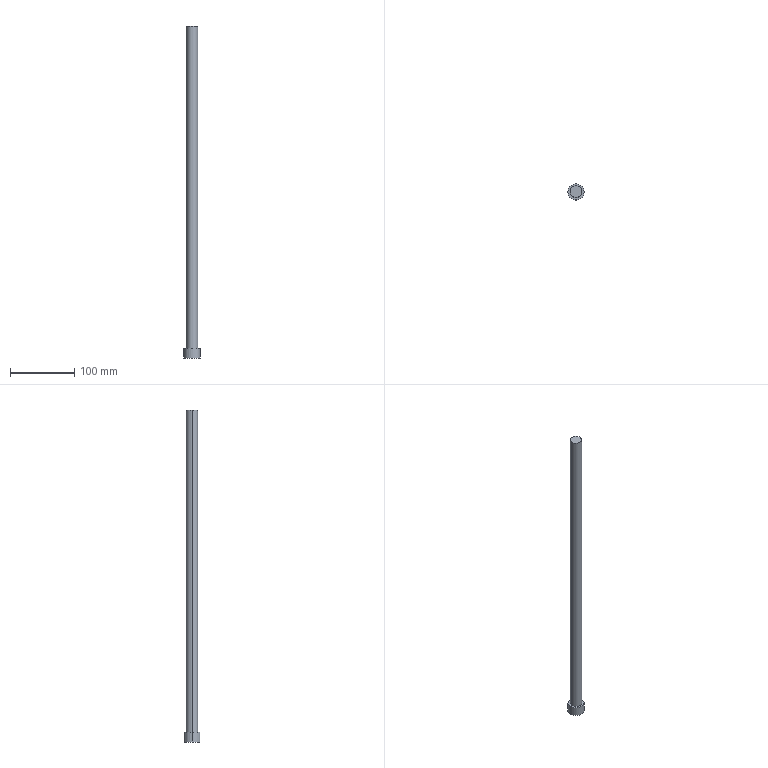Part | SolidWorks | features Extrusion 1, ICE 1 | 1 solid | 7 faces | box 25 x 25 x 515 mm | volume 134598 mm3 | cylinder 4 | plane 3 | commonest cylinder face diameters 18 x2 25 x2
STEP:
#1=CARTESIAN_POINT('',(-12.5,0.,-15.));
#2=VERTEX_POINT('',#1);
#3=CARTESIAN_POINT('',(12.5,0.,-15.));
#4=VERTEX_POINT('',#3);
#5=CARTESIAN_POINT('',(0.,0.,-15.));
#6=DIRECTION('',(0.,0.,-1.));
#7=DIRECTION('',(-1.,0.,0.));
#8=AXIS2_PLACEMENT_3D('',#5,#6,#7);
#9=CIRCLE('',#8,12.5);
#10=EDGE_CURVE('',#2,#4,#9,.T.);
#11=ORIENTED_EDGE('',*,*,#10,.F.);
#12=CARTESIAN_POINT('',(-12.5,0.,0.));
#13=VERTEX_POINT('',#12);
#14=CARTESIAN_POINT('',(-12.5,0.,-15.));
#15=DIRECTION('',(0.,0.,1.));
#16=VECTOR('',#15,1000.);
#17=LINE('',#14,#16);
#18=EDGE_CURVE('',#2,#13,#17,.T.);
#19=ORIENTED_EDGE('',*,*,#18,.T.);
#20=CARTESIAN_POINT('',(12.5,0.,0.));
#21=VERTEX_POINT('',#20);
#22=CARTESIAN_POINT('',(0.,0.,0.));
#23=DIRECTION('',(0.,0.,-1.));
#24=DIRECTION('',(-1.,0.,0.));
#25=AXIS2_PLACEMENT_3D('',#22,#23,#24);
#26=CIRCLE('',#25,12.5);
#27=EDGE_CURVE('',#13,#21,#26,.T.);
#28=ORIENTED_EDGE('',*,*,#27,.T.);
#29=CARTESIAN_POINT('',(12.5,0.,-15.));
#30=DIRECTION('',(0.,0.,1.));
#31=VECTOR('',#30,1000.);
#32=LINE('',#29,#31);
#33=EDGE_CURVE('',#4,#21,#32,.T.);
#34=ORIENTED_EDGE('',*,*,#33,.F.);
#35=EDGE_LOOP('',(#11,#19,#28,#34));
#36=FACE_OUTER_BOUND('',#35,.T.);
#37=CARTESIAN_POINT('',(0.,0.,-15.));
#38=DIRECTION('',(0.,0.,1.));
#39=DIRECTION('',(1.,0.,0.));
#40=AXIS2_PLACEMENT_3D('',#37,#38,#39);
#41=CYLINDRICAL_SURFACE('',#40,12.5);
#42=ADVANCED_FACE('',(#36),#41,.T.);
#43=CARTESIAN_POINT('',(9.,0.,500.));
#44=VERTEX_POINT('',#43);
#45=CARTESIAN_POINT('',(-9.,0.,500.));
#46=VERTEX_POINT('',#45);
#47=CARTESIAN_POINT('',(0.,0.,500.));
#48=DIRECTION('',(0.,0.,1.));
#49=DIRECTION('',(1.,0.,0.));
#50=AXIS2_PLACEMENT_3D('',#47,#48,#49);
#51=CIRCLE('',#50,9.);
#52=EDGE_CURVE('',#44,#46,#51,.T.);
#53=ORIENTED_EDGE('',*,*,#52,.F.);
#54=CARTESIAN_POINT('',(9.,0.,0.));
#55=VERTEX_POINT('',#54);
#56=CARTESIAN_POINT('',(9.,0.,500.));
#57=DIRECTION('',(0.,0.,-1.));
#58=VECTOR('',#57,1000.);
#59=LINE('',#56,#58);
#60=EDGE_CURVE('',#44,#55,#59,.T.);
#61=ORIENTED_EDGE('',*,*,#60,.T.);
#62=CARTESIAN_POINT('',(-9.,0.,0.));
#63=VERTEX_POINT('',#62);
#64=CARTESIAN_POINT('',(0.,0.,0.));
#65=DIRECTION('',(0.,0.,-1.));
#66=DIRECTION('',(-1.,0.,0.));
#67=AXIS2_PLACEMENT_3D('',#64,#65,#66);
#68=CIRCLE('',#67,9.);
#69=EDGE_CURVE('',#63,#55,#68,.T.);
#70=ORIENTED_EDGE('',*,*,#69,.F.);
#71=CARTESIAN_POINT('',(-9.,0.,500.));
#72=DIRECTION('',(0.,0.,-1.));
#73=VECTOR('',#72,1000.);
#74=LINE('',#71,#73);
#75=EDGE_CURVE('',#46,#63,#74,.T.);
#76=ORIENTED_EDGE('',*,*,#75,.F.);
#77=EDGE_LOOP('',(#53,#61,#70,#76));
#78=FACE_OUTER_BOUND('',#77,.T.);
#79=CARTESIAN_POINT('',(0.,0.,500.));
#80=DIRECTION('',(0.,0.,-1.));
#81=DIRECTION('',(-1.,0.,0.));
#82=AXIS2_PLACEMENT_3D('',#79,#80,#81);
#83=CYLINDRICAL_SURFACE('',#82,9.);
#84=ADVANCED_FACE('',(#78),#83,.T.);
#85=ORIENTED_EDGE('',*,*,#60,.F.);
#86=CARTESIAN_POINT('',(0.,0.,500.));
#87=DIRECTION('',(0.,0.,1.));
#88=DIRECTION('',(1.,0.,0.));
#89=AXIS2_PLACEMENT_3D('',#86,#87,#88);
#90=CIRCLE('',#89,9.);
#91=EDGE_CURVE('',#46,#44,#90,.T.);
#92=ORIENTED_EDGE('',*,*,#91,.F.);
#93=ORIENTED_EDGE('',*,*,#75,.T.);
#94=CARTESIAN_POINT('',(0.,0.,0.));
#95=DIRECTION('',(0.,0.,-1.));
#96=DIRECTION('',(-1.,0.,0.));
#97=AXIS2_PLACEMENT_3D('',#94,#95,#96);
#98=CIRCLE('',#97,9.);
#99=EDGE_CURVE('',#55,#63,#98,.T.);
#100=ORIENTED_EDGE('',*,*,#99,.F.);
#101=EDGE_LOOP('',(#85,#92,#93,#100));
#102=FACE_OUTER_BOUND('',#101,.T.);
#103=CARTESIAN_POINT('',(0.,0.,500.));
#104=DIRECTION('',(0.,0.,-1.));
#105=DIRECTION('',(-1.,0.,0.));
#106=AXIS2_PLACEMENT_3D('',#103,#104,#105);
#107=CYLINDRICAL_SURFACE('',#106,9.);
#108=ADVANCED_FACE('',(#102),#107,.T.);
#109=ORIENTED_EDGE('',*,*,#91,.T.);
#110=ORIENTED_EDGE('',*,*,#52,.T.);
#111=EDGE_LOOP('',(#109,#110));
#112=FACE_OUTER_BOUND('',#111,.T.);
#113=CARTESIAN_POINT('',(0.,0.,500.));
#114=DIRECTION('',(0.,0.,1.));
#115=DIRECTION('',(1.,0.,0.));
#116=AXIS2_PLACEMENT_3D('',#113,#114,#115);
#117=PLANE('',#116);
#118=ADVANCED_FACE('',(#112),#117,.T.);
#119=ORIENTED_EDGE('',*,*,#18,.F.);
#120=CARTESIAN_POINT('',(0.,0.,-15.));
#121=DIRECTION('',(0.,0.,-1.));
#122=DIRECTION('',(-1.,0.,0.));
#123=AXIS2_PLACEMENT_3D('',#120,#121,#122);
#124=CIRCLE('',#123,12.5);
#125=EDGE_CURVE('',#4,#2,#124,.T.);
#126=ORIENTED_EDGE('',*,*,#125,.F.);
#127=ORIENTED_EDGE('',*,*,#33,.T.);
#128=CARTESIAN_POINT('',(0.,0.,0.));
#129=DIRECTION('',(0.,0.,-1.));
#130=DIRECTION('',(-1.,0.,0.));
#131=AXIS2_PLACEMENT_3D('',#128,#129,#130);
#132=CIRCLE('',#131,12.5);
#133=EDGE_CURVE('',#21,#13,#132,.T.);
#134=ORIENTED_EDGE('',*,*,#133,.T.);
#135=EDGE_LOOP('',(#119,#126,#127,#134));
#136=FACE_OUTER_BOUND('',#135,.T.);
#137=CARTESIAN_POINT('',(0.,0.,-15.));
#138=DIRECTION('',(0.,0.,1.));
#139=DIRECTION('',(1.,0.,0.));
#140=AXIS2_PLACEMENT_3D('',#137,#138,#139);
#141=CYLINDRICAL_SURFACE('',#140,12.5);
#142=ADVANCED_FACE('',(#136),#141,.T.);
#143=ORIENTED_EDGE('',*,*,#125,.T.);
#144=ORIENTED_EDGE('',*,*,#10,.T.);
#145=EDGE_LOOP('',(#143,#144));
#146=FACE_OUTER_BOUND('',#145,.T.);
#147=CARTESIAN_POINT('',(0.,0.,-15.));
#148=DIRECTION('',(0.,0.,-1.));
#149=DIRECTION('',(-1.,0.,0.));
#150=AXIS2_PLACEMENT_3D('',#147,#148,#149);
#151=PLANE('',#150);
#152=ADVANCED_FACE('',(#146),#151,.T.);
#153=ORIENTED_EDGE('',*,*,#69,.T.);
#154=ORIENTED_EDGE('',*,*,#99,.T.);
#155=EDGE_LOOP('',(#153,#154));
#156=FACE_BOUND('',#155,.T.);
#157=ORIENTED_EDGE('',*,*,#133,.F.);
#158=ORIENTED_EDGE('',*,*,#27,.F.);
#159=EDGE_LOOP('',(#157,#158));
#160=FACE_OUTER_BOUND('',#159,.T.);
#161=CARTESIAN_POINT('',(0.,0.,0.));
#162=DIRECTION('',(0.,0.,-1.));
#163=DIRECTION('',(-1.,0.,0.));
#164=AXIS2_PLACEMENT_3D('',#161,#162,#163);
#165=PLANE('',#164);
#166=ADVANCED_FACE('',(#156,#160),#165,.F.);
#167=CLOSED_SHELL('',(#42,#84,#108,#118,#142,#152,#166));
#168=MANIFOLD_SOLID_BREP('',#167);
#169=CARTESIAN_POINT('',(0.,0.,0.));
#170=DIRECTION('',(0.,0.,1.));
#171=DIRECTION('',(1.,0.,0.));
#172=AXIS2_PLACEMENT_3D('',#169,#170,#171);
#173=(LENGTH_UNIT()NAMED_UNIT(*)SI_UNIT(.MILLI.,.METRE.));
#174=UNCERTAINTY_MEASURE_WITH_UNIT(LENGTH_MEASURE(0.00001),#173,'','');
#175=(NAMED_UNIT(*)PLANE_ANGLE_UNIT()SI_UNIT($,.RADIAN.));
#176=(NAMED_UNIT(*)SI_UNIT($,.STERADIAN.)SOLID_ANGLE_UNIT());
#177=(GEOMETRIC_REPRESENTATION_CONTEXT(3)GLOBAL_UNCERTAINTY_ASSIGNED_CONTEXT((#174))GLOBAL_UNIT_ASSIGNED_CONTEXT((#173,#175,#176))REPRESENTATION_CONTEXT('',''));
#178=ADVANCED_BREP_SHAPE_REPRESENTATION('',(#168,#172),#177);